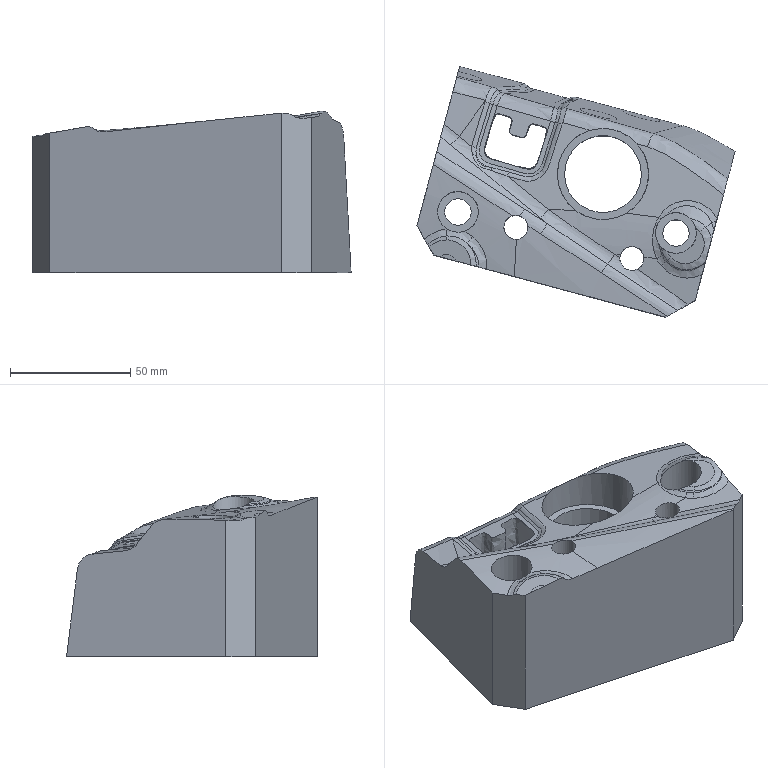Part | NX | features solid 2 | 1 solid | 94 faces | box 132.517 x 104.515 x 67.268 mm | volume 394513 mm3 | spline 75 | plane 10 | cylinder 9 | commonest cylinder face diameters 10 x2 11 x2 17 x2 32 x1 38 x1 41 x1